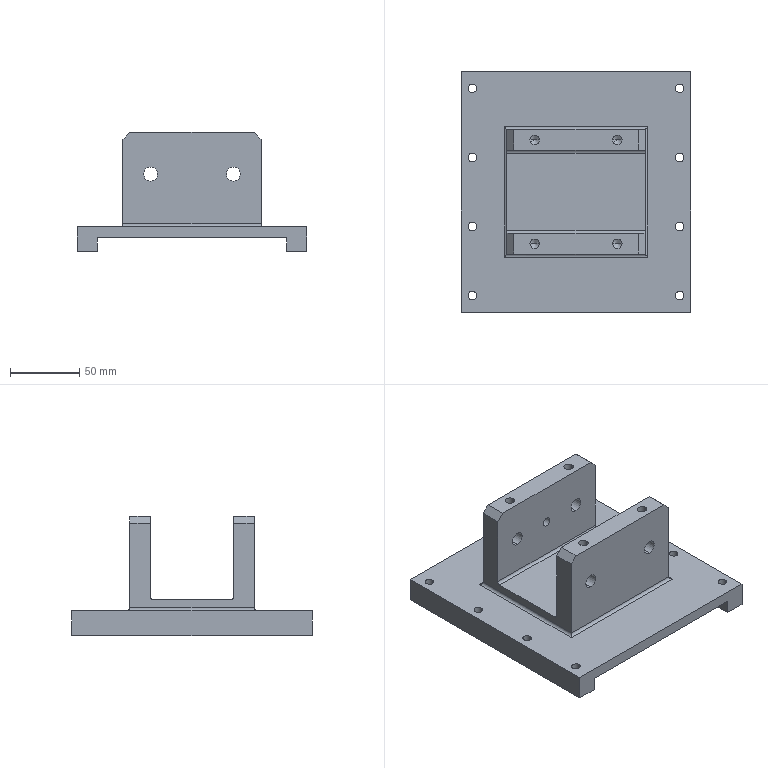NC program | NX | posted with a generic post | part box 166 x 174 x 86.2 mm
Lines 1 to 1226 of 4531:
N10 G17 G21 G94 G90
(PLANAR_MILL_1 , TOOL : D16-48-D16-100-3T-FINISH)
N12 T02 M6
N14 G53
N16 G17 G0 G90 X-22.05 Y63. B0. C0. S2000 M3
N18 G43 Z30. H2
N20 Z-7.7
N22 G94 G1 Z-9.7 F800.
N24 Y50.
N26 Y-50.
N28 Y-63.
N30 Z-7.7
N32 G0 Z30.
N34 X22.05
N36 Z-7.7
N38 G1 Z-9.7
N40 Y-50.
N42 Y50.
N44 Y63.
N46 Z-7.7
N48 G0 Z30.
N50 X-22.05
N52 Z-17.4
N54 G1 Z-19.4
N56 Y50.
N58 Y-50.
N60 Y-63.
N62 Z-17.4
N64 G0 Z30.
N66 X22.05
N68 Z-17.4
N70 G1 Z-19.4
N72 Y-50.
N74 Y50.
N76 Y63.
N78 Z-17.4
N80 G0 Z30.
N82 X-22.05
N84 Z-27.1
N86 G1 Z-29.1
N88 Y50.
N90 Y-50.
N92 Y-63.
N94 Z-27.1
N96 G0 Z30.
N98 X22.05
N100 Z-27.1
N102 G1 Z-29.1
N104 Y-50.
N106 Y50.
N108 Y63.
N110 Z-27.1
N112 G0 Z30.
N114 X-22.05
N116 Z-36.8
N118 G1 Z-38.8
N120 Y50.
N122 Y-50.
N124 Y-63.
N126 Z-36.8
N128 G0 Z30.
N130 X22.05
N132 Z-36.8
N134 G1 Z-38.8
N136 Y-50.
N138 Y50.
N140 Y63.
N142 Z-36.8
N144 G0 Z30.
N146 X-22.05
N148 Z-46.5
N150 G1 Z-48.5
N152 Y50.
N154 Y-50.
N156 Y-63.
N158 Z-46.5
N160 G0 Z30.
N162 X22.05
N164 Z-46.5
N166 G1 Z-48.5
N168 Y-50.
N170 Y50.
N172 Y63.
N174 Z-46.5
N176 G0 Z30.
N178 X-22.05
N180 Z-56.2
N182 G1 Z-58.2
N184 Y50.
N186 Y-50.
N188 Y-63.
N190 Z-56.2
N192 G0 Z30.
N194 X22.05
N196 Z-56.2
N198 G1 Z-58.2
N200 Y-50.
N202 Y50.
N204 Y63.
N206 Z-56.2
N208 G0 Z30.
(PLANAR_MILL_1_COPY , TOOL : D16-48-D16-100-3T-FINISH)
N210 X-22.1
N212 Z-56.2
N214 G1 Z-58.2
N216 Y50.
N218 Y-50.
N220 Y-63.
N222 Z-56.2
N224 G0 Z30.
N226 Y63.
N228 Z-56.2
N230 G1 Z-58.2
N232 Y50.
N234 Y-50.
N236 Y-63.
N238 Z-56.2
N240 G0 Z30.
N242 X22.1
N244 Z-56.2
N246 G1 Z-58.2
N248 Y-50.
N250 Y50.
N252 Y63.
N254 Z-56.2
N256 G0 Z30.
N258 Y-63.
N260 Z-56.2
N262 G1 Z-58.2
N264 Y-50.
N266 Y50.
N268 Y63.
N270 Z-56.2
N272 G0 Z30.
(PLANAR_MILL , TOOL : D16-48-D16-100-3T-FINISH)
N274 X53.15 Y60.258
N276 Z-7.457
N278 G1 Z-9.457
N280 Y49.998
N282 Y-50.
N284 G2 X45.1 Y-58.05 R8.05
N286 G1 X-45.1
N288 G2 X-53.15 Y-50. R8.05
N290 G1 Y50.
N292 G2 X-45.1 Y58.05 R8.05
N294 G1 X45.098
N296 X55.358
N298 Z-7.457
N300 G0 Z30.
N302 X53.15 Y60.258
N304 Z-7.457
N306 G1 Z-9.457
N308 Y49.998
N310 Y-50.
N312 G2 X45.1 Y-58.05 R8.05
N314 G1 X-45.1
N316 G2 X-53.15 Y-50. R8.05
N318 G1 Y50.
N320 G2 X-45.1 Y58.05 R8.05
N322 G1 X45.098
N324 X55.358
N326 Z-7.457
N328 G0 Z30.
N330 X53.15 Y60.258
N332 Z-16.914
N334 G1 Z-18.914
N336 Y49.998
N338 Y-50.
N340 G2 X45.1 Y-58.05 R8.05
N342 G1 X-45.1
N344 G2 X-53.15 Y-50. R8.05
N346 G1 Y50.
N348 G2 X-45.1 Y58.05 R8.05
N350 G1 X45.098
N352 X55.358
N354 Z-16.914
N356 G0 Z30.
N358 X53.15 Y60.258
N360 Z-16.914
N362 G1 Z-18.914
N364 Y49.998
N366 Y-50.
N368 G2 X45.1 Y-58.05 R8.05
N370 G1 X-45.1
N372 G2 X-53.15 Y-50. R8.05
N374 G1 Y50.
N376 G2 X-45.1 Y58.05 R8.05
N378 G1 X45.098
N380 X55.358
N382 Z-16.914
N384 G0 Z30.
N386 X53.15 Y60.258
N388 Z-26.371
N390 G1 Z-28.371
N392 Y49.998
N394 Y-50.
N396 G2 X45.1 Y-58.05 R8.05
N398 G1 X-45.1
N400 G2 X-53.15 Y-50. R8.05
N402 G1 Y50.
N404 G2 X-45.1 Y58.05 R8.05
N406 G1 X45.098
N408 X55.358
N410 Z-26.371
N412 G0 Z30.
N414 X53.15 Y60.258
N416 Z-26.371
N418 G1 Z-28.371
N420 Y49.998
N422 Y-50.
N424 G2 X45.1 Y-58.05 R8.05
N426 G1 X-45.1
N428 G2 X-53.15 Y-50. R8.05
N430 G1 Y50.
N432 G2 X-45.1 Y58.05 R8.05
N434 G1 X45.098
N436 X55.358
N438 Z-26.371
N440 G0 Z30.
N442 X53.15 Y60.258
N444 Z-35.829
N446 G1 Z-37.829
N448 Y49.998
N450 Y-50.
N452 G2 X45.1 Y-58.05 R8.05
N454 G1 X-45.1
N456 G2 X-53.15 Y-50. R8.05
N458 G1 Y50.
N460 G2 X-45.1 Y58.05 R8.05
N462 G1 X45.098
N464 X55.358
N466 Z-35.829
N468 G0 Z30.
N470 X53.15 Y60.258
N472 Z-35.829
N474 G1 Z-37.829
N476 Y49.998
N478 Y-50.
N480 G2 X45.1 Y-58.05 R8.05
N482 G1 X-45.1
N484 G2 X-53.15 Y-50. R8.05
N486 G1 Y50.
N488 G2 X-45.1 Y58.05 R8.05
N490 G1 X45.098
N492 X55.358
N494 Z-35.829
N496 G0 Z30.
N498 X53.15 Y60.258
N500 Z-45.286
N502 G1 Z-47.286
N504 Y49.998
N506 Y-50.
N508 G2 X45.1 Y-58.05 R8.05
N510 G1 X-45.1
N512 G2 X-53.15 Y-50. R8.05
N514 G1 Y50.
N516 G2 X-45.1 Y58.05 R8.05
N518 G1 X45.098
N520 X55.358
N522 Z-45.286
N524 G0 Z30.
N526 X53.15 Y60.258
N528 Z-45.286
N530 G1 Z-47.286
N532 Y49.998
N534 Y-50.
N536 G2 X45.1 Y-58.05 R8.05
N538 G1 X-45.1
N540 G2 X-53.15 Y-50. R8.05
N542 G1 Y50.
N544 G2 X-45.1 Y58.05 R8.05
N546 G1 X45.098
N548 X55.358
N550 Z-45.286
N552 G0 Z30.
N554 X53.15 Y60.258
N556 Z-54.743
N558 G1 Z-56.743
N560 Y49.998
N562 Y-50.
N564 G2 X45.1 Y-58.05 R8.05
N566 G1 X-45.1
N568 G2 X-53.15 Y-50. R8.05
N570 G1 Y50.
N572 G2 X-45.1 Y58.05 R8.05
N574 G1 X45.098
N576 X55.358
N578 Z-54.743
N580 G0 Z30.
N582 X53.15 Y60.258
N584 Z-54.743
N586 G1 Z-56.743
N588 Y49.998
N590 Y-50.
N592 G2 X45.1 Y-58.05 R8.05
N594 G1 X-45.1
N596 G2 X-53.15 Y-50. R8.05
N598 G1 Y50.
N600 G2 X-45.1 Y58.05 R8.05
N602 G1 X45.098
N604 X55.358
N606 Z-54.743
N608 G0 Z30.
N610 X53.15 Y60.258
N612 Z-64.2
N614 G1 Z-66.2
N616 Y49.998
N618 Y-50.
N620 G2 X45.1 Y-58.05 R8.05
N622 G1 X-45.1
N624 G2 X-53.15 Y-50. R8.05
N626 G1 Y50.
N628 G2 X-45.1 Y58.05 R8.05
N630 G1 X45.098
N632 X55.358
N634 Z-64.2
N636 G0 Z30.
N638 X53.15 Y60.258
N640 Z-64.2
N642 G1 Z-66.2
N644 Y49.998
N646 Y-50.
N648 G2 X45.1 Y-58.05 R8.05
N650 G1 X-45.1
N652 G2 X-53.15 Y-50. R8.05
N654 G1 Y50.
N656 G2 X-45.1 Y58.05 R8.05
N658 G1 X45.098
N660 X55.358
N662 Z-64.2
N664 G0 Z30.
(PLANAR_MILL_COPY , TOOL : D16-48-D16-100-3T-FINISH)
N666 X53.1 Y60.247
N668 Z-64.2
N670 G1 Z-66.2
N672 Y49.998
N674 Y-50.
N676 G2 X45.1 Y-58. R8.
N678 G1 X-45.1
N680 G2 X-53.1 Y-50. R8.
N682 G1 Y50.
N684 G2 X-45.1 Y58. R8.
N686 G1 X45.098
N688 X55.347
N690 Z-64.2
N692 G0 Z30.
N694 X53.1 Y60.247
N696 Z-64.2
N698 G1 Z-66.2
N700 Y49.998
N702 Y-50.
N704 G2 X45.1 Y-58. R8.
N706 G1 X-45.1
N708 G2 X-53.1 Y-50. R8.
N710 G1 Y50.
N712 G2 X-45.1 Y58. R8.
N714 G1 X45.098
N716 X55.347
N718 Z-64.2
N720 G0 Z30.
(FLOOR_WALL , TOOL : D16-48-D16-100-3T-FINISH)
N722 X-4. Y61.
N724 Z-57.15
N726 G1 Z-60.15
N728 Y50.
N730 G3 X0. Y46. R4.
N732 G1 X20.544
N734 Y-46.
N736 X-20.544
N738 Y46.
N740 X0.
N742 Y34.
N744 X8.544
N746 Y-34.
N748 X-8.544
N750 Y34.
N752 X0.
N754 Y26.8
N756 X1.344
N758 Y-26.8
N760 X-1.344
N762 Y26.8
N764 X0.
N766 X1.
N768 G3 X5. Y30.8 R4.
N770 G1 Z-57.15
N772 G0 Z30.
(FLOOR_WALL_COPY_1 , TOOL : D16-48-D16-100-3T-FINISH)
N774 X-4. Y61.
N776 Z-57.2
N778 G1 Z-60.2
N780 Y50.
N782 G3 X0. Y46. R4.
N784 G1 X20.344
N786 Y-46.
N788 X-20.344
N790 Y46.
N792 X0.
N794 Y34.
N796 X8.344
N798 Y-34.
N800 X-8.344
N802 Y34.
N804 X0.
N806 Y26.8
N808 X1.144
N810 Y-26.8
N812 X-1.144
N814 Y26.8
N816 X0.
N818 X1.
N820 G3 X5. Y30.8 R4.
N822 G1 Z-57.2
N824 G0 Z30.
(FLOOR_WALL_COPY , TOOL : D16-48-D16-100-3T-FINISH)
N826 X-98. Y-4.
N828 Z-65.15
N830 G1 Z-68.15
N832 X-87.
N834 G3 X-83. Y0. R4.
N836 G1 Y79.
N838 X83.
N840 Y-79.
N842 X-83.
N844 Y0.
N846 X-71.
N848 Y67.
N850 X71.
N852 Y-67.
N854 X55.456
N856 Y-55.
N858 Y55.
N860 X59.
N862 Y-55.
N864 X55.456
N866 Y-67.
N868 X-71.
N870 Y0.
N872 X-59.
N874 Y55.
N876 X-55.456
N878 Y-55.
N880 X-59.
N882 Y0.
N884 X-58.656 Y-4.
N886 G3 X-54.656 Y0. R4.
N888 G1 Y59.556
N890 X54.656
N892 Y-59.556
N894 X-54.656
N896 Y0.
N898 Y1.
N900 G3 X-58.656 Y5. R4.
N902 G1 Z-65.15
N904 G0 Z30.
(FLOOR_WALL_COPY_COPY , TOOL : D16-48-D16-100-3T-FINISH)
N906 X-98. Y-4.
N908 Z-65.2
N910 G1 Z-68.2
N912 X-87.
N914 G3 X-83. Y0. R4.
N916 G1 Y79.
N918 X83.
N920 Y-79.
N922 X-83.
N924 Y0.
N926 X-71.
N928 Y67.
N930 X71.
N932 Y-67.
N934 X55.656
N936 Y-55.
N938 Y55.
N940 X59.
N942 Y-55.
N944 X55.656
N946 Y-67.
N948 X-71.
N950 Y0.
N952 X-59.
N954 Y55.
N956 X-55.656
N958 Y-55.
N960 X-59.
N962 Y0.
N964 X-58.856 Y-4.
N966 G3 X-54.856 Y0. R4.
N968 G1 Y59.756
N970 X54.856
N972 Y-59.756
N974 X-54.856
N976 Y0.
N978 Y1.
N980 G3 X-58.856 Y5. R4.
N982 G1 Z-65.2
N984 G0 Z30.
(AREA_MILL , TOOL : D16-48-D16-100-3T-FINISH)
N986 X-55.05 Y-59.949 S3500
N988 Z-60.199
N990 G1 Y-59.911 Z-60.983 F2000.
N992 Y-59.796 Z-61.759
N994 Y-59.605 Z-62.521
N996 Y-59.34 Z-63.26
N998 Y-59.005 Z-63.97
N1000 Y-58.601 Z-64.643
N1002 Y-58.134 Z-65.274
N1004 Y-57.606 Z-65.855
N1006 Y-57.025 Z-66.383
N1008 Y-56.394 Z-66.85
N1010 Y-55.721 Z-67.254
N1012 Y-55.011 Z-67.59
N1014 Y-54.272 Z-67.854
N1016 Y-53.51 Z-68.045
N1018 Y-52.734 Z-68.16
N1020 Y-51.949 Z-68.199
N1022 Y51.95 Z-68.198
N1024 X-55. Y51.9 Z-68.196
N1026 Y-51.9
N1028 X-54.95 Y-51.85 Z-68.191
N1030 Y51.85
N1032 X-54.901 Y51.801 Z-68.187
N1034 Y-51.801
N1036 X-54.851 Y-51.751 Z-68.183
N1038 Y51.751
N1040 X-54.821 Y51.721 Z-68.181
N1042 X-54.801 Y51.701 Z-68.177
N1044 Y-51.701
N1046 X-54.752 Y-51.652 Z-68.167
N1048 Y24.516 Z-68.166
N1050 Y51.652 Z-68.167
N1052 X-54.703 Y51.604 Z-68.158
N1054 Y-32.401 Z-68.156
N1056 Y-51.604 Z-68.158
N1058 X-54.654 Y-51.556 Z-68.149
N1060 Y-3.582 Z-68.146
N1062 Y51.555 Z-68.149
N1064 X-54.606 Y51.507 Z-68.138
N1066 Y51.35 Z-68.136
N1068 Y-23.286 Z-68.134
N1070 Y-51.348 Z-68.136
N1072 Y-51.508 Z-68.138
N1074 X-54.558 Y-51.459 Z-68.124
N1076 Y-51.35 Z-68.122
N1078 Y15.798 Z-68.12
N1080 Y51.35 Z-68.122
N1082 Y51.459 Z-68.124
N1084 X-54.511 Y51.412 Z-68.109
N1086 Y3.573 Z-68.105
N1088 Y-51.412 Z-68.109
N1090 X-54.463 Y-51.364 Z-68.094
N1092 Y24.481 Z-68.091
N1094 Y51.364 Z-68.093
N1096 X-54.416 Y51.317 Z-68.077
N1098 Y15.41 Z-68.075
N1100 Y-17.908 Z-68.077
N1102 Y-51.316
N1104 X-54.37 Y-51.269 Z-68.058
N1106 Y-13.136 Z-68.056
N1108 Y-12.65 Z-68.061
N1110 Y15.039 Z-68.059
N1112 Y15.525 Z-68.055
N1114 Y51.27 Z-68.059
N1116 X-54.324 Y51.225 Z-68.04
N1118 Y15.525 Z-68.036
N1120 Y14.789 Z-68.043
N1122 Y-12.4
N1124 Y-13.136 Z-68.036
N1126 Y-51.224 Z-68.039
N1128 X-54.28 Y-51.181 Z-68.02
N1130 Y-13.136 Z-68.016
N1132 Y-12.761 Z-68.02
N1134 Y15.15 Z-68.021
N1136 Y15.525 Z-68.018
N1138 Y51.182 Z-68.021
N1140 X-54.236 Y51.139 Z-68.003
N1142 Y-22.688 Z-67.996
N1144 Y-51.138 Z-68.002
N1146 X-54.192 Y-51.094 Z-67.978
N1148 Y-13.235 Z-67.974
N1150 Y51.095 Z-67.979
N1152 X-54.148 Y51.051 Z-67.955
N1154 Y-26.073 Z-67.951
N1156 Y-51.05 Z-67.954
N1158 X-54.105 Y-51.008 Z-67.931
N1160 Y-50.553 Z-67.929
N1162 Y6.835 Z-67.928
N1164 Y51.008 Z-67.93
N1166 X-54.061 Y50.966 Z-67.906
N1168 Y-50.645 Z-67.905
N1170 Y-50.966 Z-67.908
N1172 X-54.038 Y-50.944 Z-67.896
N1174 X-54.019 Y-50.924 Z-67.882
N1176 Y-50.553 Z-67.878
N1178 Y-9.951
N1180 Y-9.791 Z-67.879
N1182 Y36.044 Z-67.88
N1184 Y50.924
N1186 X-53.979 Y50.882 Z-67.851
N1188 Y50.723
N1190 Y50.656 Z-67.853
N1192 Y50.627 Z-67.851
N1194 Y44.981 Z-67.85
N1196 Y44.496 Z-67.853
N1198 Y36.099
N1200 Y36.044 Z-67.851
N1202 Y21.097 Z-67.85
N1204 Y20.613 Z-67.853
N1206 Y-9.466
N1208 Y-9.951 Z-67.848
N1210 Y-50.675 Z-67.85
N1212 Y-50.796 Z-67.855
N1214 Y-50.883
N1216 X-53.959 Y-50.862 Z-67.841
N1218 X-53.94 Y-50.843 Z-67.826
N1220 Y-50.755 Z-67.822
N1222 Y-9.951 Z-67.819
N1224 Y-9.155 Z-67.826
N1226 Y20.309
N1228 Y21.097 Z-67.822
N1230 Y36.044 Z-67.823
N1232 Y36.134 Z-67.826
N1234 Y44.193
N1236 Y44.981 Z-67.823
N1238 Y50.626
N1240 Y50.675 Z-67.826
N1242 Y50.722 Z-67.823
N1244 Y50.843
N1246 X-53.901 Y50.806 Z-67.795
N1248 Y50.721
N1250 Y50.654 Z-67.797
N1252 Y50.625 Z-67.795
N1254 Y44.981
N1256 Y44.507 Z-67.797
N1258 Y36.097
N1260 Y36.044 Z-67.795
N1262 Y21.097 Z-67.794
N1264 Y20.624 Z-67.797
N1266 Y-9.477 Z-67.794
N1268 Y-9.951 Z-67.79
N1270 Y-50.553 Z-67.793
N1272 Y-50.805 Z-67.795
N1274 X-53.862 Y-50.767 Z-67.766
N1276 Y-9.951 Z-67.761
N1278 Y-9.792 Z-67.762
N1280 Y40.442 Z-67.768
N1282 Y50.769
N1284 X-53.835 Y50.743 Z-67.747
N1286 X-53.824 Y50.732 Z-67.737
N1288 Y21.277 Z-67.735
N1290 Y-9.234 Z-67.73
N1292 Y-9.314 Z-67.732
N1294 Y-36.065 Z-67.735
N1296 Y-36.223 Z-67.733
N1298 Y-50.553 Z-67.734
N1300 Y-50.628 Z-67.738
N1302 Y-50.731
N1304 X-53.804 Y-50.711 Z-67.723
N1306 X-53.788 Y-50.694 Z-67.708
N1308 Y-50.553 Z-67.701
N1310 Y-36.223 Z-67.699
N1312 Y-35.749 Z-67.705
N1314 Y-9.629 Z-67.702
N1316 Y-9.392 Z-67.698
N1318 Y39.607 Z-67.703
N1320 Y49.758
N1322 Y50.596 Z-67.706
N1324 Y50.693 Z-67.705
N1326 X-53.752 Y50.657 Z-67.673
N1328 Y50.52 Z-67.674
N1330 Y49.758 Z-67.671
N1332 Y22.889 Z-67.67
N1334 Y-9.547 Z-67.666
N1336 Y-9.938 Z-67.674
N1338 Y-35.44 Z-67.676
N1340 Y-36.223 Z-67.667
N1342 Y-50.553 Z-67.669
N1344 Y-50.656 Z-67.673
N1346 X-53.716 Y-50.622 Z-67.64
N1348 Y-50.553 Z-67.637
N1350 Y-36.223 Z-67.635
N1352 Y-35.717 Z-67.641
N1354 Y-9.951 Z-67.64
N1356 Y-9.698 Z-67.635
N1358 Y46.374 Z-67.639
N1360 Y49.758
N1362 Y50.624 Z-67.642
N1364 X-53.681 Y50.589 Z-67.609
N1366 Y49.758 Z-67.607
N1368 Y-9.849 Z-67.604
N1370 Y-9.951 Z-67.606
N1372 Y-36.019 Z-67.605
N1374 Y-36.223 Z-67.603
N1376 Y-50.553 Z-67.605
N1378 Y-50.587 Z-67.606
N1380 X-53.647 Y-50.553 Z-67.572
N1382 Y-31.994 Z-67.569
N1384 Y50.555 Z-67.574
N1386 X-53.616 Y50.52 Z-67.537
N1388 Y28.622 Z-67.535
N1390 Y28.262 Z-67.534
N1392 Y-42.592 Z-67.532
N1394 Y-50.518 Z-67.534
N1396 X-53.584 Y-50.482 Z-67.496
N1398 Y-28.461 Z-67.494
N1400 Y28.262 Z-67.495
N1402 Y28.893 Z-67.498
N1404 Y50.485 Z-67.5
N1406 X-53.553 Y50.454 Z-67.462
N1408 Y28.953 Z-67.459
N1410 Y28.262 Z-67.456
N1412 Y-49.757 Z-67.457
N1414 Y-50.452 Z-67.458
N1416 X-53.522 Y-50.423 Z-67.421
N1418 Y-45.777 Z-67.419
N1420 Y28.262 Z-67.418
N1422 Y28.687 Z-67.42
N1424 Y50.425 Z-67.424
N1426 X-53.491 Y50.396 Z-67.385
N1428 Y24.381 Z-67.38
N1430 Y-49.839 Z-67.382
N1432 Y-50.395 Z-67.384
N1434 X-53.461 Y-50.368 Z-67.347
N1436 Y-49.757 Z-67.343
N1438 Y23.568 Z-67.341
N1440 Y49.758 Z-67.344
N1442 Y50.368 Z-67.348
N1444 X-53.436 Y50.34 Z-67.308
N1446 Y49.758 Z-67.305
N1448 Y-20.423 Z-67.299
N1450 Y-49.757 Z-67.303
N1452 Y-50.34 Z-67.307
N1454 X-53.41 Y-50.312 Z-67.267
N1456 Y-49.757 Z-67.262
N1458 Y-14.728 Z-67.256
N1460 Y45.045 Z-67.264
N1462 Y49.758 Z-67.265
N1464 Y50.312 Z-67.269
N1466 X-53.384 Y50.284 Z-67.229
N1468 Y49.758 Z-67.225
N1470 Y24.182 Z-67.223
N1472 Y-17.116 Z-67.213
N1474 Y-49.757 Z-67.222
N1476 Y-50.285 Z-67.227
N1478 Y-51.069 Z-67.195
N1480 Y-51.847 Z-67.086
N1482 Y-52.61 Z-66.902
N1484 Y-53.351 Z-66.644
N1486 Y-54.064 Z-66.314
N1488 Y-54.74 Z-65.916
N1490 Y-55.375 Z-65.454
N1492 Y-55.961 Z-64.932
N1494 Y-56.493 Z-64.355
N1496 Y-56.967 Z-63.728
N1498 Y-57.376 Z-63.058
N1500 Y-57.718 Z-62.352
N1502 Y-57.988 Z-61.615
N1504 Y-58.186 Z-60.855
N1506 Y-58.308 Z-60.079
N1508 Y-58.353 Z-59.295
N1510 G0 Z30.
(AREA_MILL_COPY , TOOL : D16-48-D16-100-3T-FINISH)
N1512 X-55.05 Y59.95
N1514 Z-60.198
N1516 G1 X-55.012 Z-60.983
N1518 X-54.896 Z-61.759
N1520 X-54.706 Z-62.521
N1522 X-54.441 Z-63.26
N1524 X-54.106 Z-63.97
N1526 X-53.702 Z-64.643
N1528 X-53.234 Z-65.274
N1530 X-52.707 Z-65.855
N1532 X-52.125 Z-66.383
N1534 X-51.495 Z-66.85
N1536 X-50.821 Z-67.254
N1538 X-50.112 Z-67.589
N1540 X-49.372 Z-67.854
N1542 X-48.611 Z-68.045
N1544 X-47.834 Z-68.16
N1546 X-47.05 Z-68.198
N1548 X47.05
N1550 X47. Y59.9 Z-68.196
N1552 X-47.
N1554 X-46.951 Y59.85 Z-68.191
N1556 X46.95
N1558 X46.901 Y59.801 Z-68.187
N1560 X-2.978 Z-68.186
N1562 X-46.901 Z-68.187
N1564 X-46.851 Y59.751 Z-68.183
N1566 X19.439 Z-68.18
N1568 X46.851 Z-68.183
N1570 X46.822 Y59.721 Z-68.18
N1572 X46.802 Y59.701 Z-68.177
N1574 X0.8 Z-68.174
N1576 X-46.802 Z-68.177
N1578 X-46.752 Y59.652 Z-68.167
N1580 X19.859 Z-68.165
N1582 X46.752 Z-68.167
N1584 X46.704 Y59.603 Z-68.158
N1586 X-18.16 Z-68.155
N1588 X-46.704 Z-68.158
N1590 X-46.655 Y59.554 Z-68.149
N1592 X-6. Z-68.146
N1594 X46.655 Z-68.149
N1596 X46.607 Y59.506 Z-68.138
N1598 X46.336 Z-68.136
N1600 X-25.4 Z-68.135
N1602 X-46.4 Z-68.136
N1604 X-46.607 Z-68.138
N1606 X-46.559 Y59.458 Z-68.124
N1608 X-46.4 Z-68.122
N1610 X16.669 Z-68.12
N1612 X46.335 Z-68.122
N1614 X46.359 Z-68.124
N1616 X46.559 Z-68.125
N1618 X46.512 Y59.41 Z-68.111
N1620 X46.355 Z-68.109
N1622 X46.333 Z-68.107
N1624 X-3.883 Z-68.106
N1626 X-46.4 Z-68.107
N1628 X-46.511 Z-68.109
N1630 X-46.464 Y59.363 Z-68.094
N1632 X21.183 Z-68.091
N1634 X46.343 Z-68.094
N1636 X46.389 Z-68.095
N1638 X46.4 Z-68.094
N1640 X46.464 Z-68.095
N1642 X46.417 Y59.316 Z-68.078
N1644 X12.8 Z-68.075
N1646 X-19.8 Z-68.077
N1648 X-46.417 Z-68.078
N1650 X-46.37 Y59.27 Z-68.059
N1652 X-16. Z-68.056
N1654 X-15.515 Z-68.061
N1656 X13.115 Z-68.06
N1658 X13.6 Z-68.055
N1660 X46.37 Z-68.059
N1662 X46.324 Y59.225 Z-68.04
N1664 X13.6 Z-68.036
N1666 X12.857 Z-68.043
N1668 X-15.258
N1670 X-16. Z-68.036
N1672 X-46.324 Z-68.04
N1674 X-46.282 Y59.181 Z-68.022
N1676 X-16. Z-68.016
N1678 X-15.62 Z-68.02
N1680 X13.219 Z-68.021
N1682 X13.6 Z-68.018
N1684 X46.281 Z-68.022
N1686 X46.239 Y59.136 Z-68.003
N1688 X-20.099 Z-67.997
N1690 X-46.24 Z-68.004
N1692 X-46.196 Y59.092 Z-67.98
N1694 X-13.94 Z-67.974
N1696 X46.195 Z-67.979
N1698 X46.151 Y59.049 Z-67.955
N1700 X-19.957 Z-67.951
N1702 X-46.152 Z-67.956
N1704 X-46.109 Y59.005 Z-67.932
N1706 X-45.6 Z-67.931
N1708 X-2.514 Z-67.928
N1710 X46.108 Z-67.931
N1712 X46.066 Y58.962 Z-67.906
N1714 X12.064 Z-67.904
N1716 X-45.676 Z-67.906
N1718 X-46.067 Z-67.908
N1720 X-46.026 Y58.919 Z-67.883
N1722 X-45.6 Z-67.88
N1724 X32.8 Z-67.879
N1726 X40.643 Z-67.88
N1728 X46.025
N1730 X45.983 Y58.879 Z-67.852
N1732 X45.764 Z-67.853
N1734 X45.74 Z-67.851
N1736 X40.8
N1738 X40.314 Z-67.853
N1740 X38.085
N1742 X37.6 Z-67.851
N1744 X9.6 Z-67.85
N1746 X-45.746 Z-67.852
N1748 X-45.843 Z-67.855
N1750 X-45.985 Z-67.856
N1752 X-45.945 Y58.84 Z-67.828
N1754 X-45.842 Z-67.824
N1756 X-40.968 Z-67.823
N1758 X37.6
N1760 X38.4 Z-67.826
N1762 X40.007
N1764 X40.8 Z-67.823
N1766 X45.723
N1768 X45.763 Z-67.826
N1770 X45.944
N1772 X45.905 Y58.8 Z-67.796
N1774 X45.729
N1776 X45.706 Z-67.794
N1778 X40.8
N1780 X40.332 Z-67.796
N1782 X38.067
N1784 X37.6 Z-67.794
N1786 X-45.6
N1788 X-45.905 Z-67.796
N1790 X-45.867 Y58.76 Z-67.767
N1792 X-45.6 Z-67.766
N1794 X45.867
N1796 X45.829 Y58.722 Z-67.735
N1798 X-32.617
N1800 X-41.8 Z-67.734
N1802 X-45.6 Z-67.735
N1804 X-45.829 Z-67.736
N1806 X-45.792 Y58.685 Z-67.704
N1808 X-44.8 Z-67.701
N1810 X-32.8 Z-67.7
N1812 X-32.301 Z-67.703
N1814 X16.3
N1816 X16.8 Z-67.701
N1818 X28.
N1820 X28.03 Z-67.703
N1822 X28.066
N1824 X28.096 Z-67.701
N1826 X28.117 Z-67.703
N1828 X28.141
N1830 X28.162 Z-67.701
N1832 X28.182 Z-67.703
N1834 X28.207
N1836 X28.227 Z-67.701
N1838 X28.244 Z-67.703
N1840 X28.265
N1842 X28.283 Z-67.701
N1844 X28.3 Z-67.703
N1846 X28.321
N1848 X28.338 Z-67.701
N1850 X28.8
N1852 X28.812 Z-67.703
N1854 X28.842 Z-67.701
N1856 X28.869 Z-67.703
N1858 X28.902
N1860 X28.929 Z-67.701
N1862 X28.949 Z-67.703
N1864 X28.972
N1866 X28.991 Z-67.701
N1868 X29.011 Z-67.703
N1870 X29.034
N1872 X29.053 Z-67.701
N1874 X44.8
N1876 X45.632 Z-67.703
N1878 X45.791
N1880 X45.754 Y58.648 Z-67.671
N1882 X45.669 Z-67.67
N1884 X45.6 Z-67.671
N1886 X44.8 Z-67.668
N1888 X29.056
N1890 X29.024 Z-67.671
N1892 X28.994 Z-67.668
N1894 X28.962 Z-67.671
N1896 X28.932 Z-67.668
N1898 X28.887 Z-67.671
N1900 X28.844 Z-67.668
N1902 X28.82 Z-67.671
N1904 X28.8 Z-67.668
N1906 X28.338
N1908 X28.31 Z-67.671
N1910 X28.283 Z-67.668
N1912 X28.254 Z-67.671
N1914 X28.227 Z-67.668
N1916 X28.194 Z-67.671
N1918 X28.162 Z-67.668
N1920 X28.128 Z-67.671
N1922 X28.096 Z-67.668
N1924 X28.047 Z-67.671
N1926 X28. Z-67.668
N1928 X16.8
N1930 X16.016 Z-67.671
N1932 X-32.016
N1934 X-32.8 Z-67.666
N1936 X-44.8 Z-67.668
N1938 X-45.754 Z-67.672
N1940 X-45.721 Y58.613 Z-67.64
N1942 X-45.6 Z-67.637
N1944 X-44.8 Z-67.635
N1946 X-32.8 Z-67.633
N1948 X-32.323 Z-67.636
N1950 X16.322 Z-67.638
N1952 X16.8 Z-67.635
N1954 X28.
N1956 X28.029 Z-67.638
N1958 X28.068
N1960 X28.096 Z-67.635
N1962 X28.116 Z-67.638
N1964 X28.142
N1966 X28.162 Z-67.635
N1968 X28.181 Z-67.638
N1970 X28.208
N1972 X28.227 Z-67.635
N1974 X28.244 Z-67.638
N1976 X28.266
N1978 X28.283 Z-67.635
N1980 X28.299 Z-67.638
N1982 X28.321
N1984 X28.338 Z-67.635
N1986 X28.8
N1988 X28.811 Z-67.638
N1990 X28.831
N1992 X28.846 Z-67.635
N1994 X28.873 Z-67.638
N1996 X28.908
N1998 X28.934 Z-67.635
N2000 X28.952 Z-67.638
N2002 X28.977
N2004 X28.996 Z-67.635
N2006 X29.014 Z-67.638
N2008 X29.039
N2010 X29.058 Z-67.635
N2012 X44.8
N2014 X45.6 Z-67.637
N2016 X45.72 Z-67.638
N2018 X45.686 Y58.577 Z-67.605
N2020 X45.659 Z-67.603
N2022 X45.638 Z-67.605
N2024 X45.6 Z-67.604
N2026 X-29.477 Z-67.601
N2028 X-29.553 Z-67.603
N2030 X-29.6 Z-67.601
N2032 X-35.8
N2034 X-45.6 Z-67.604
N2036 X-45.686 Z-67.605
N2038 X-45.653 Y58.544 Z-67.572
N2040 X-45.6 Z-67.57
N2042 X-29.48 Z-67.566
N2044 X45.603 Z-67.57
N2046 X45.65 Z-67.566
N2048 X45.618 Y58.513 Z-67.533
N2050 X29.984 Z-67.532
N2052 X29.6 Z-67.53
N2054 X-32. Z-67.528
N2056 X-32.385 Z-67.53
N2058 X-45.619 Z-67.534
N2060 X-45.584 Y58.482 Z-67.496
N2062 X-32.656 Z-67.494
N2064 X-32. Z-67.491
N2066 X-29.519 Z-67.492
N2068 X29.6 Z-67.491
N2070 X30.255 Z-67.495
N2072 X45.584 Z-67.496
N2074 X45.551 Y58.45 Z-67.458
N2076 X30.273 Z-67.456
N2078 X29.6 Z-67.452
N2080 X-29.49 Z-67.454
N2082 X-29.577 Z-67.455
N2084 X-29.6 Z-67.454
N2086 X-32.
N2088 X-32.673 Z-67.457
N2090 X-45.551 Z-67.459
N2092 X-45.519 Y58.42 Z-67.42
N2094 X-32.409 Z-67.419
N2096 X-32. Z-67.417
N2098 X-29.6
N2100 X-29.552 Z-67.42
N2102 X-29.493 Z-67.417
N2104 X25.6 Z-67.415
N2106 X29.6 Z-67.414
N2108 X30.009 Z-67.417
N2110 X45.519 Z-67.42
N2112 X45.49 Y58.389 Z-67.382
N2114 X26.95 Z-67.377
N2116 X-26.4 Z-67.381
N2118 X-29.496
N2120 X-29.548 Z-67.383
N2122 X-29.566 Z-67.382
N2124 X-29.574 Z-67.383
N2126 X-29.6 Z-67.381
N2128 X-45.491 Z-67.382
N2130 X-45.464 Y58.362 Z-67.347
N2132 X-44.8 Z-67.345
N2134 X-29.596 Z-67.344
N2136 X-29.569 Z-67.34
N2138 X-29.51 Z-67.344
N2140 X-13.6
N2142 X-13.418 Z-67.346
N2144 X8.618 Z-67.344
N2146 X8.8 Z-67.342
N2148 X30.4 Z-67.34
N2150 X44.8 Z-67.345
N2152 X45.464 Z-67.347
N2154 X45.437 Y58.336 Z-67.308
N2156 X44.8 Z-67.305
N2158 X22. Z-67.302
N2160 X8.8
N2162 X8.177 Z-67.308
N2164 X-12.977
N2166 X-13.6 Z-67.301
N2168 X-29.54 Z-67.303
N2170 X-29.571 Z-67.301
N2172 X-29.586 Z-67.303
N2174 X-44.8 Z-67.306
N2176 X-45.437 Z-67.308
N2178 X-45.41 Y58.311 Z-67.269
N2180 X-44.8 Z-67.267
N2182 X-13.6 Z-67.258
N2184 X-13.059 Z-67.265
N2186 X8.259 Z-67.267
N2188 X8.8 Z-67.262
N2190 X45.097 Z-67.268
N2192 X45.409 Z-67.269
N2194 X45.384 Y58.287 Z-67.233
N2196 X44.8 Z-67.23
N2198 X22.6 Z-67.229
N2200 X8.8 Z-67.225
N2202 X5.899 Z-67.226
N2204 X-13.465 Z-67.221
N2206 X-13.6 Z-67.219
N2208 X-29.243 Z-67.224
N2210 X-29.245 Z-67.223
N2212 X-29.269 Z-67.224
N2214 X-29.526
N2216 X-29.576 Z-67.222
N2218 X-29.593 Z-67.224
N2220 X-44.874 Z-67.231
N2222 X-45.384 Z-67.233
N2224 X-46.169 Z-67.199
N2226 X-46.946 Z-67.089
N2228 X-47.709 Z-66.902
N2230 X-48.449 Z-66.642
N2232 X-49.161 Z-66.31
N2234 X-49.837 Z-65.91
N2236 X-50.47 Z-65.446
N2238 X-51.054 Z-64.922
N2240 X-51.585 Z-64.344
N2242 X-52.056 Z-63.716
N2244 X-52.464 Z-63.045
N2246 X-52.803 Z-62.337
N2248 X-53.072 Z-61.599
N2250 X-53.267 Z-60.839
N2252 X-53.387 Z-60.063
N2254 X-53.429 Z-59.279
N2256 G0 Z30.
(AREA_MILL_COPY_COPY , TOOL : D16-48-D16-100-3T-FINISH)
N2258 X55.05 Y59.95
N2260 Z-60.198
N2262 G1 Y59.911 Z-60.983
N2264 Y59.796 Z-61.759
N2266 Y59.605 Z-62.521
N2268 Y59.341 Z-63.26
N2270 Y59.005 Z-63.97
N2272 Y58.601 Z-64.643
N2274 Y58.134 Z-65.274
N2276 Y57.607 Z-65.855
N2278 Y57.025 Z-66.383
N2280 Y56.394 Z-66.85
N2282 Y55.721 Z-67.254
N2284 Y55.011 Z-67.59
N2286 Y54.272 Z-67.854
N2288 Y53.51 Z-68.045
N2290 Y52.734 Z-68.16
N2292 Y51.95 Z-68.198
N2294 Y-51.949 Z-68.199
N2296 X55. Y-51.9 Z-68.196
N2298 Y51.9
N2300 X54.95 Y51.85 Z-68.191
N2302 Y-51.85
N2304 X54.901 Y-51.801 Z-68.187
N2306 Y51.801
N2308 X54.851 Y51.751 Z-68.183
N2310 Y-51.751
N2312 X54.821 Y-51.722 Z-68.181
N2314 X54.801 Y-51.702 Z-68.177
N2316 Y51.702
N2318 X54.752 Y51.652 Z-68.167
N2320 Y-51.652
N2322 X54.703 Y-51.604 Z-68.158
N2324 Y51.604
N2326 X54.654 Y51.555 Z-68.149
N2328 Y-51.555
N2330 X54.605 Y-51.507 Z-68.138
N2332 Y-51.35 Z-68.136
N2334 Y51.349
N2336 Y51.507 Z-68.138
N2338 X54.558 Y51.459 Z-68.124
N2340 Y51.348 Z-68.122
N2342 Y-51.35
N2344 Y-51.459 Z-68.124
N2346 X54.51 Y-51.411 Z-68.109
N2348 Y-10.747 Z-68.107
N2350 Y51.411 Z-68.108
N2352 X54.462 Y51.363 Z-68.093
N2354 Y-44.782
N2356 Y-51.363
N2358 X54.415 Y-51.315 Z-68.077
N2360 Y-9.982 Z-68.076
N2362 Y51.316 Z-68.077
N2364 X54.369 Y51.269 Z-68.058
N2366 Y-51.102 Z-68.057
N2368 Y-51.268 Z-68.058
N2370 X54.323 Y-51.222 Z-68.038
N2372 Y51.223 Z-68.039
N2374 X54.277 Y51.179 Z-68.02
N2376 Y-51.178 Z-68.019
N2378 X54.231 Y-51.133 Z-67.999
N2380 Y51.134 Z-68.001
N2382 X54.187 Y51.09 Z-67.976
N2384 Y-51.089 Z-67.975
N2386 X54.144 Y-51.045 Z-67.952
N2388 Y51.046
N2390 X54.1 Y51.004 Z-67.928